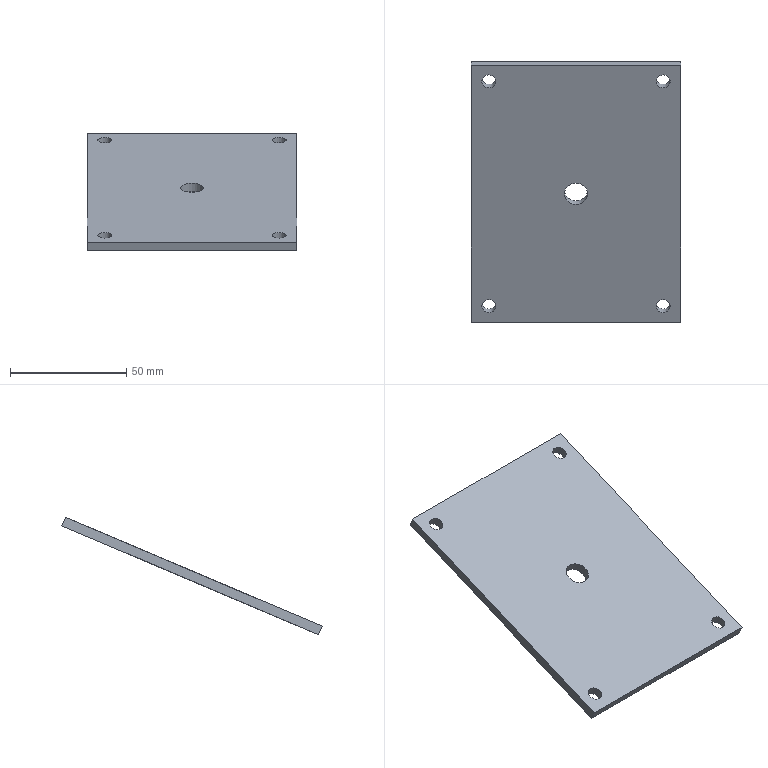Part | NX | features SIMPLE HOLE 57, DATUM_CSYS 28, HOLE PACKAGE 27, SKETCH 27, EXTRUDE 18, EXTRACT_FACE 16, EXTRACT_DATUM_AXIS 10, BLEND 8, CBORE_HOLE 7, EXTRACT_DATUM_PLANE 6, FSET 6, Instance Feature 5, Mirror Feature 5, DRAFT 4, EXTRACT_STRING 2, DELETE FACE 1, OFFSET_REGION 1 | 1 solid | 11 faces | box 90 x 112.024 x 50.57 mm | volume 42433 mm3 | plane 6 | cylinder 5 | commonest cylinder face diameters 6 x4 10 x1
STEP:
#1=CARTESIAN_POINT('',(-45.,-38.214,107.268));
#2=VERTEX_POINT('',#1);
#3=CARTESIAN_POINT('',(-45.,72.246,154.156));
#4=VERTEX_POINT('',#3);
#5=CARTESIAN_POINT('',(-45.,72.246,154.156));
#6=DIRECTION('',(0.,0.9205,0.3907));
#7=VECTOR('',#6,1000.);
#8=LINE('',#5,#7);
#9=EDGE_CURVE('',#2,#4,#8,.T.);
#10=ORIENTED_EDGE('',*,*,#9,.F.);
#11=CARTESIAN_POINT('',(-45.,-39.777,110.95));
#12=VERTEX_POINT('',#11);
#13=CARTESIAN_POINT('',(-45.,17.27,-23.444));
#14=DIRECTION('',(0.,-0.3907,0.9205));
#15=VECTOR('',#14,1000.);
#16=LINE('',#13,#15);
#17=EDGE_CURVE('',#2,#12,#16,.T.);
#18=ORIENTED_EDGE('',*,*,#17,.T.);
#19=CARTESIAN_POINT('',(-45.,70.684,157.838));
#20=VERTEX_POINT('',#19);
#21=CARTESIAN_POINT('',(-45.,70.684,157.838));
#22=DIRECTION('',(0.,-0.9205,-0.3907));
#23=VECTOR('',#22,1000.);
#24=LINE('',#21,#23);
#25=EDGE_CURVE('',#20,#12,#24,.T.);
#26=ORIENTED_EDGE('',*,*,#25,.F.);
#27=CARTESIAN_POINT('',(-45.,127.73,23.444));
#28=DIRECTION('',(0.,-0.3907,0.9205));
#29=VECTOR('',#28,1000.);
#30=LINE('',#27,#29);
#31=EDGE_CURVE('',#4,#20,#30,.T.);
#32=ORIENTED_EDGE('',*,*,#31,.F.);
#33=EDGE_LOOP('',(#10,#18,#26,#32));
#34=FACE_BOUND('',#33,.T.);
#35=CARTESIAN_POINT('',(-45.,127.73,23.444));
#36=DIRECTION('',(1.,0.,0.));
#37=DIRECTION('',(0.,0.,-1.));
#38=AXIS2_PLACEMENT_3D('',#35,#36,#37);
#39=PLANE('',#38);
#40=ADVANCED_FACE('',(#34),#39,.F.);
#41=CARTESIAN_POINT('',(45.,72.246,154.156));
#42=VERTEX_POINT('',#41);
#43=CARTESIAN_POINT('',(45.,-38.214,107.268));
#44=VERTEX_POINT('',#43);
#45=CARTESIAN_POINT('',(45.,72.246,154.156));
#46=DIRECTION('',(0.,-0.9205,-0.3907));
#47=VECTOR('',#46,1000.);
#48=LINE('',#45,#47);
#49=EDGE_CURVE('',#42,#44,#48,.T.);
#50=ORIENTED_EDGE('',*,*,#49,.F.);
#51=CARTESIAN_POINT('',(45.,70.684,157.838));
#52=VERTEX_POINT('',#51);
#53=CARTESIAN_POINT('',(45.,73.028,152.315));
#54=DIRECTION('',(0.,0.3907,-0.9205));
#55=VECTOR('',#54,1000.);
#56=LINE('',#53,#55);
#57=EDGE_CURVE('',#52,#42,#56,.T.);
#58=ORIENTED_EDGE('',*,*,#57,.F.);
#59=CARTESIAN_POINT('',(45.,-39.777,110.95));
#60=VERTEX_POINT('',#59);
#61=CARTESIAN_POINT('',(45.,70.684,157.838));
#62=DIRECTION('',(0.,-0.9205,-0.3907));
#63=VECTOR('',#62,1000.);
#64=LINE('',#61,#63);
#65=EDGE_CURVE('',#52,#60,#64,.T.);
#66=ORIENTED_EDGE('',*,*,#65,.T.);
#67=CARTESIAN_POINT('',(45.,-37.433,105.427));
#68=DIRECTION('',(0.,0.3907,-0.9205));
#69=VECTOR('',#68,1000.);
#70=LINE('',#67,#69);
#71=EDGE_CURVE('',#60,#44,#70,.T.);
#72=ORIENTED_EDGE('',*,*,#71,.T.);
#73=EDGE_LOOP('',(#50,#58,#66,#72));
#74=FACE_BOUND('',#73,.T.);
#75=CARTESIAN_POINT('',(45.,73.028,152.315));
#76=DIRECTION('',(-1.,0.,0.));
#77=DIRECTION('',(0.,0.,1.));
#78=AXIS2_PLACEMENT_3D('',#75,#76,#77);
#79=PLANE('',#78);
#80=ADVANCED_FACE('',(#74),#79,.F.);
#81=ORIENTED_EDGE('',*,*,#57,.T.);
#82=CARTESIAN_POINT('',(0.,72.246,154.156));
#83=DIRECTION('',(-1.,0.,0.));
#84=VECTOR('',#83,1000.);
#85=LINE('',#82,#84);
#86=EDGE_CURVE('',#42,#4,#85,.T.);
#87=ORIENTED_EDGE('',*,*,#86,.T.);
#88=ORIENTED_EDGE('',*,*,#31,.T.);
#89=CARTESIAN_POINT('',(-45.,70.684,157.838));
#90=DIRECTION('',(1.,0.,0.));
#91=VECTOR('',#90,1000.);
#92=LINE('',#89,#91);
#93=EDGE_CURVE('',#20,#52,#92,.T.);
#94=ORIENTED_EDGE('',*,*,#93,.T.);
#95=EDGE_LOOP('',(#81,#87,#88,#94));
#96=FACE_BOUND('',#95,.T.);
#97=CARTESIAN_POINT('',(0.,116.662,49.52));
#98=DIRECTION('',(0.,0.9205,0.3907));
#99=DIRECTION('',(0.,-0.3907,0.9205));
#100=AXIS2_PLACEMENT_3D('',#97,#98,#99);
#101=PLANE('',#100);
#102=ADVANCED_FACE('',(#96),#101,.T.);
#103=CARTESIAN_POINT('',(0.,-38.214,107.268));
#104=DIRECTION('',(-1.,0.,0.));
#105=VECTOR('',#104,1000.);
#106=LINE('',#103,#105);
#107=EDGE_CURVE('',#44,#2,#106,.T.);
#108=ORIENTED_EDGE('',*,*,#107,.F.);
#109=ORIENTED_EDGE('',*,*,#71,.F.);
#110=CARTESIAN_POINT('',(-45.,-39.777,110.95));
#111=DIRECTION('',(1.,0.,0.));
#112=VECTOR('',#111,1000.);
#113=LINE('',#110,#112);
#114=EDGE_CURVE('',#12,#60,#113,.T.);
#115=ORIENTED_EDGE('',*,*,#114,.F.);
#116=ORIENTED_EDGE('',*,*,#17,.F.);
#117=EDGE_LOOP('',(#108,#109,#115,#116));
#118=FACE_BOUND('',#117,.T.);
#119=CARTESIAN_POINT('',(0.,6.201,2.632));
#120=DIRECTION('',(0.,0.9205,0.3907));
#121=DIRECTION('',(0.,-0.3907,0.9205));
#122=AXIS2_PLACEMENT_3D('',#119,#120,#121);
#123=PLANE('',#122);
#124=ADVANCED_FACE('',(#118),#123,.F.);
#125=CARTESIAN_POINT('',(-37.5,-30.112,115.053));
#126=VERTEX_POINT('',#125);
#127=CARTESIAN_POINT('',(-37.5,-32.873,113.88));
#128=DIRECTION('',(0.,0.3907,-0.9205));
#129=DIRECTION('',(0.,0.9205,0.3907));
#130=AXIS2_PLACEMENT_3D('',#127,#128,#129);
#131=CIRCLE('',#130,3.);
#132=EDGE_CURVE('',#126,#126,#131,.T.);
#133=ORIENTED_EDGE('',*,*,#132,.F.);
#134=EDGE_LOOP('',(#133));
#135=FACE_BOUND('',#134,.T.);
#136=CARTESIAN_POINT('',(-37.5,-28.549,111.37));
#137=VERTEX_POINT('',#136);
#138=CARTESIAN_POINT('',(-37.5,-31.31,110.198));
#139=DIRECTION('',(0.,0.3907,-0.9205));
#140=DIRECTION('',(0.,0.9205,0.3907));
#141=AXIS2_PLACEMENT_3D('',#138,#139,#140);
#142=CIRCLE('',#141,3.);
#143=EDGE_CURVE('',#137,#137,#142,.F.);
#144=ORIENTED_EDGE('',*,*,#143,.F.);
#145=EDGE_LOOP('',(#144));
#146=FACE_BOUND('',#145,.T.);
#147=CARTESIAN_POINT('',(-37.5,-30.529,108.357));
#148=DIRECTION('',(0.,0.3907,-0.9205));
#149=DIRECTION('',(0.,0.9205,0.3907));
#150=AXIS2_PLACEMENT_3D('',#147,#148,#149);
#151=CYLINDRICAL_SURFACE('',#150,3.);
#152=ADVANCED_FACE('',(#135,#146),#151,.F.);
#153=CARTESIAN_POINT('',(-37.5,66.541,156.079));
#154=VERTEX_POINT('',#153);
#155=CARTESIAN_POINT('',(-37.5,63.78,154.907));
#156=DIRECTION('',(0.,0.3907,-0.9205));
#157=DIRECTION('',(0.,0.9205,0.3907));
#158=AXIS2_PLACEMENT_3D('',#155,#156,#157);
#159=CIRCLE('',#158,3.);
#160=EDGE_CURVE('',#154,#154,#159,.T.);
#161=ORIENTED_EDGE('',*,*,#160,.F.);
#162=EDGE_LOOP('',(#161));
#163=FACE_BOUND('',#162,.T.);
#164=CARTESIAN_POINT('',(-37.5,68.104,152.397));
#165=VERTEX_POINT('',#164);
#166=CARTESIAN_POINT('',(-37.5,65.343,151.225));
#167=DIRECTION('',(0.,0.3907,-0.9205));
#168=DIRECTION('',(0.,0.9205,0.3907));
#169=AXIS2_PLACEMENT_3D('',#166,#167,#168);
#170=CIRCLE('',#169,3.);
#171=EDGE_CURVE('',#165,#165,#170,.F.);
#172=ORIENTED_EDGE('',*,*,#171,.F.);
#173=EDGE_LOOP('',(#172));
#174=FACE_BOUND('',#173,.T.);
#175=CARTESIAN_POINT('',(-37.5,66.124,149.384));
#176=DIRECTION('',(0.,0.3907,-0.9205));
#177=DIRECTION('',(0.,0.9205,0.3907));
#178=AXIS2_PLACEMENT_3D('',#175,#176,#177);
#179=CYLINDRICAL_SURFACE('',#178,3.);
#180=ADVANCED_FACE('',(#163,#174),#179,.F.);
#181=CARTESIAN_POINT('',(37.5,-30.112,115.053));
#182=VERTEX_POINT('',#181);
#183=CARTESIAN_POINT('',(37.5,-32.873,113.88));
#184=DIRECTION('',(0.,0.3907,-0.9205));
#185=DIRECTION('',(0.,0.9205,0.3907));
#186=AXIS2_PLACEMENT_3D('',#183,#184,#185);
#187=CIRCLE('',#186,3.);
#188=EDGE_CURVE('',#182,#182,#187,.T.);
#189=ORIENTED_EDGE('',*,*,#188,.F.);
#190=EDGE_LOOP('',(#189));
#191=FACE_BOUND('',#190,.T.);
#192=CARTESIAN_POINT('',(37.5,-28.549,111.37));
#193=VERTEX_POINT('',#192);
#194=CARTESIAN_POINT('',(37.5,-31.31,110.198));
#195=DIRECTION('',(0.,0.3907,-0.9205));
#196=DIRECTION('',(0.,0.9205,0.3907));
#197=AXIS2_PLACEMENT_3D('',#194,#195,#196);
#198=CIRCLE('',#197,3.);
#199=EDGE_CURVE('',#193,#193,#198,.F.);
#200=ORIENTED_EDGE('',*,*,#199,.F.);
#201=EDGE_LOOP('',(#200));
#202=FACE_BOUND('',#201,.T.);
#203=CARTESIAN_POINT('',(37.5,-30.529,108.357));
#204=DIRECTION('',(0.,0.3907,-0.9205));
#205=DIRECTION('',(0.,0.9205,0.3907));
#206=AXIS2_PLACEMENT_3D('',#203,#204,#205);
#207=CYLINDRICAL_SURFACE('',#206,3.);
#208=ADVANCED_FACE('',(#191,#202),#207,.F.);
#209=CARTESIAN_POINT('',(37.5,66.541,156.079));
#210=VERTEX_POINT('',#209);
#211=CARTESIAN_POINT('',(37.5,63.78,154.907));
#212=DIRECTION('',(0.,0.3907,-0.9205));
#213=DIRECTION('',(0.,0.9205,0.3907));
#214=AXIS2_PLACEMENT_3D('',#211,#212,#213);
#215=CIRCLE('',#214,3.);
#216=EDGE_CURVE('',#210,#210,#215,.T.);
#217=ORIENTED_EDGE('',*,*,#216,.F.);
#218=EDGE_LOOP('',(#217));
#219=FACE_BOUND('',#218,.T.);
#220=CARTESIAN_POINT('',(37.5,68.104,152.397));
#221=VERTEX_POINT('',#220);
#222=CARTESIAN_POINT('',(37.5,65.343,151.225));
#223=DIRECTION('',(0.,0.3907,-0.9205));
#224=DIRECTION('',(0.,0.9205,0.3907));
#225=AXIS2_PLACEMENT_3D('',#222,#223,#224);
#226=CIRCLE('',#225,3.);
#227=EDGE_CURVE('',#221,#221,#226,.F.);
#228=ORIENTED_EDGE('',*,*,#227,.F.);
#229=EDGE_LOOP('',(#228));
#230=FACE_BOUND('',#229,.T.);
#231=CARTESIAN_POINT('',(37.5,66.124,149.384));
#232=DIRECTION('',(0.,0.3907,-0.9205));
#233=DIRECTION('',(0.,0.9205,0.3907));
#234=AXIS2_PLACEMENT_3D('',#231,#232,#233);
#235=CYLINDRICAL_SURFACE('',#234,3.);
#236=ADVANCED_FACE('',(#219,#230),#235,.F.);
#237=CARTESIAN_POINT('',(0.,20.056,136.347));
#238=VERTEX_POINT('',#237);
#239=CARTESIAN_POINT('',(0.,15.453,134.394));
#240=DIRECTION('',(0.,0.3907,-0.9205));
#241=DIRECTION('',(0.,0.9205,0.3907));
#242=AXIS2_PLACEMENT_3D('',#239,#240,#241);
#243=CIRCLE('',#242,5.);
#244=EDGE_CURVE('',#238,#238,#243,.T.);
#245=ORIENTED_EDGE('',*,*,#244,.T.);
#246=EDGE_LOOP('',(#245));
#247=FACE_BOUND('',#246,.T.);
#248=ORIENTED_EDGE('',*,*,#216,.T.);
#249=EDGE_LOOP('',(#248));
#250=FACE_BOUND('',#249,.T.);
#251=ORIENTED_EDGE('',*,*,#188,.T.);
#252=EDGE_LOOP('',(#251));
#253=FACE_BOUND('',#252,.T.);
#254=ORIENTED_EDGE('',*,*,#160,.T.);
#255=EDGE_LOOP('',(#254));
#256=FACE_BOUND('',#255,.T.);
#257=ORIENTED_EDGE('',*,*,#132,.T.);
#258=EDGE_LOOP('',(#257));
#259=FACE_BOUND('',#258,.T.);
#260=ORIENTED_EDGE('',*,*,#114,.T.);
#261=ORIENTED_EDGE('',*,*,#65,.F.);
#262=ORIENTED_EDGE('',*,*,#93,.F.);
#263=ORIENTED_EDGE('',*,*,#25,.T.);
#264=EDGE_LOOP('',(#260,#261,#262,#263));
#265=FACE_BOUND('',#264,.T.);
#266=CARTESIAN_POINT('',(-45.,70.684,157.838));
#267=DIRECTION('',(0.,0.3907,-0.9205));
#268=DIRECTION('',(0.,0.9205,0.3907));
#269=AXIS2_PLACEMENT_3D('',#266,#267,#268);
#270=PLANE('',#269);
#271=ADVANCED_FACE('',(#247,#250,#253,#256,#259,#265),#270,.F.);
#272=CARTESIAN_POINT('',(0.,21.619,132.665));
#273=VERTEX_POINT('',#272);
#274=CARTESIAN_POINT('',(0.,17.016,130.712));
#275=DIRECTION('',(0.,0.3907,-0.9205));
#276=DIRECTION('',(0.,0.9205,0.3907));
#277=AXIS2_PLACEMENT_3D('',#274,#275,#276);
#278=CIRCLE('',#277,5.);
#279=EDGE_CURVE('',#273,#273,#278,.T.);
#280=ORIENTED_EDGE('',*,*,#279,.F.);
#281=EDGE_LOOP('',(#280));
#282=FACE_BOUND('',#281,.T.);
#283=ORIENTED_EDGE('',*,*,#49,.T.);
#284=ORIENTED_EDGE('',*,*,#107,.T.);
#285=ORIENTED_EDGE('',*,*,#9,.T.);
#286=ORIENTED_EDGE('',*,*,#86,.F.);
#287=EDGE_LOOP('',(#283,#284,#285,#286));
#288=FACE_BOUND('',#287,.T.);
#289=ORIENTED_EDGE('',*,*,#143,.T.);
#290=EDGE_LOOP('',(#289));
#291=FACE_BOUND('',#290,.T.);
#292=ORIENTED_EDGE('',*,*,#171,.T.);
#293=EDGE_LOOP('',(#292));
#294=FACE_BOUND('',#293,.T.);
#295=ORIENTED_EDGE('',*,*,#199,.T.);
#296=EDGE_LOOP('',(#295));
#297=FACE_BOUND('',#296,.T.);
#298=ORIENTED_EDGE('',*,*,#227,.T.);
#299=EDGE_LOOP('',(#298));
#300=FACE_BOUND('',#299,.T.);
#301=CARTESIAN_POINT('',(330.,79.427,157.204));
#302=DIRECTION('',(0.,0.3907,-0.9205));
#303=DIRECTION('',(0.,0.9205,0.3907));
#304=AXIS2_PLACEMENT_3D('',#301,#302,#303);
#305=PLANE('',#304);
#306=ADVANCED_FACE('',(#282,#288,#291,#294,#297,#300),#305,.T.);
#307=ORIENTED_EDGE('',*,*,#279,.T.);
#308=EDGE_LOOP('',(#307));
#309=FACE_BOUND('',#308,.T.);
#310=ORIENTED_EDGE('',*,*,#244,.F.);
#311=EDGE_LOOP('',(#310));
#312=FACE_BOUND('',#311,.T.);
#313=CARTESIAN_POINT('',(0.,15.453,134.394));
#314=DIRECTION('',(0.,0.3907,-0.9205));
#315=DIRECTION('',(0.,0.9205,0.3907));
#316=AXIS2_PLACEMENT_3D('',#313,#314,#315);
#317=CYLINDRICAL_SURFACE('',#316,5.);
#318=ADVANCED_FACE('',(#309,#312),#317,.F.);
#319=CLOSED_SHELL('',(#40,#80,#102,#124,#152,#180,#208,#236,#271,#306,#318));
#320=MANIFOLD_SOLID_BREP('',#319);
#321=(LENGTH_UNIT()NAMED_UNIT(*)SI_UNIT(.MILLI.,.METRE.));
#322=UNCERTAINTY_MEASURE_WITH_UNIT(LENGTH_MEASURE(0.00001),#321,'','');
#323=(NAMED_UNIT(*)PLANE_ANGLE_UNIT()SI_UNIT($,.RADIAN.));
#324=(NAMED_UNIT(*)SI_UNIT($,.STERADIAN.)SOLID_ANGLE_UNIT());
#325=(GEOMETRIC_REPRESENTATION_CONTEXT(3)GLOBAL_UNCERTAINTY_ASSIGNED_CONTEXT((#322))GLOBAL_UNIT_ASSIGNED_CONTEXT((#321,#323,#324))REPRESENTATION_CONTEXT('',''));
#326=ADVANCED_BREP_SHAPE_REPRESENTATION('',(#320),#325);